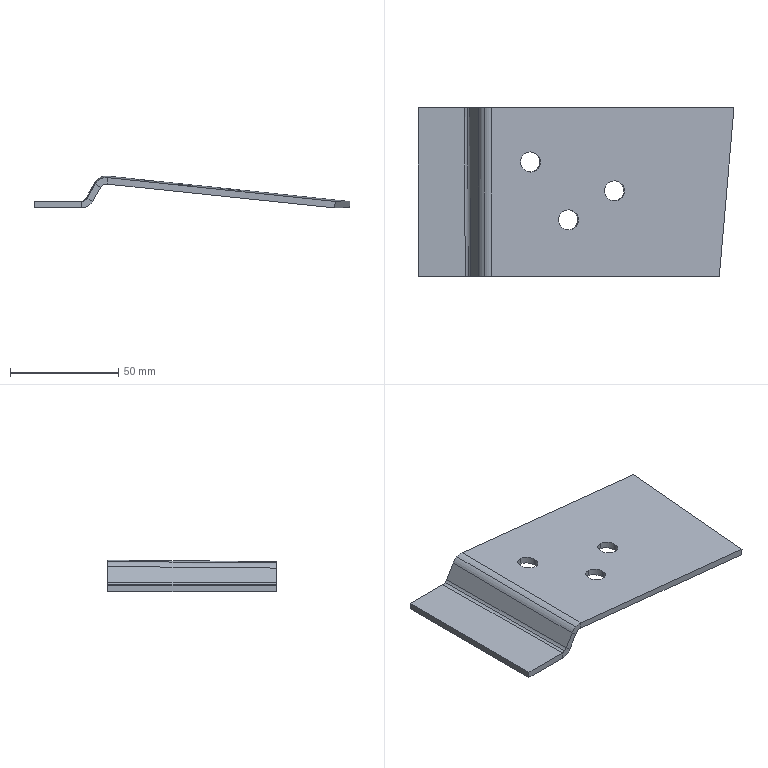Part | NX | features BREP 1 | 1 solid | 38 faces | box 145.982 x 77.757 x 14.741 mm | volume 34048 mm3 | cylinder 20 | plane 14 | spline 4 | commonest cylinder face diameters 9.3 x12 6 x4 12 x4
STEP:
#1=CARTESIAN_POINT('',(747.036,-96.197,42.475));
#2=VERTEX_POINT('',#1);
#3=CARTESIAN_POINT('',(751.661,-91.543,42.034));
#4=VERTEX_POINT('',#3);
#5=CARTESIAN_POINT('',(751.661,-91.543,42.034));
#6=CARTESIAN_POINT('',(751.661,-92.763,42.023));
#7=CARTESIAN_POINT('',(750.656,-95.185,42.106));
#8=CARTESIAN_POINT('',(748.251,-96.196,42.348));
#9=CARTESIAN_POINT('',(747.036,-96.197,42.475));
#10=B_SPLINE_CURVE_WITH_KNOTS('',3,(#5,#6,#7,#8,#9),.UNSPECIFIED.,.F.,.F.,(4,1,4),(0.,0.5,1.),.UNSPECIFIED.);
#11=EDGE_CURVE('',#2,#4,#10,.F.);
#12=ORIENTED_EDGE('',*,*,#11,.T.);
#13=CARTESIAN_POINT('',(751.348,-91.516,39.05));
#14=VERTEX_POINT('',#13);
#15=CARTESIAN_POINT('',(751.348,-91.516,39.05));
#16=DIRECTION('',(0.1041,-0.00911,0.9945));
#17=VECTOR('',#16,1000.);
#18=LINE('',#15,#17);
#19=EDGE_CURVE('',#14,#4,#18,.T.);
#20=ORIENTED_EDGE('',*,*,#19,.F.);
#21=CARTESIAN_POINT('',(746.724,-96.17,39.492));
#22=VERTEX_POINT('',#21);
#23=CARTESIAN_POINT('',(746.724,-96.17,39.492));
#24=CARTESIAN_POINT('',(747.938,-96.169,39.365));
#25=CARTESIAN_POINT('',(750.345,-95.156,39.122));
#26=CARTESIAN_POINT('',(751.348,-92.738,39.039));
#27=CARTESIAN_POINT('',(751.348,-91.516,39.05));
#28=B_SPLINE_CURVE_WITH_KNOTS('',3,(#23,#24,#25,#26,#27),.UNSPECIFIED.,.F.,.F.,(4,1,4),(0.,0.5,1.),.UNSPECIFIED.);
#29=EDGE_CURVE('',#22,#14,#28,.T.);
#30=ORIENTED_EDGE('',*,*,#29,.F.);
#31=CARTESIAN_POINT('',(746.724,-96.17,39.492));
#32=DIRECTION('',(0.1041,-0.00911,0.9945));
#33=VECTOR('',#32,1000.);
#34=LINE('',#31,#33);
#35=EDGE_CURVE('',#22,#2,#34,.T.);
#36=ORIENTED_EDGE('',*,*,#35,.T.);
#37=EDGE_LOOP('',(#12,#20,#30,#36));
#38=FACE_BOUND('',#37,.T.);
#39=CARTESIAN_POINT('',(746.724,-91.52,39.534));
#40=DIRECTION('',(0.1041,-0.00911,0.9945));
#41=DIRECTION('',(0.,-1.,-0.00916));
#42=AXIS2_PLACEMENT_3D('',#39,#40,#41);
#43=CYLINDRICAL_SURFACE('',#42,4.65);
#44=ADVANCED_FACE('',(#38),#43,.F.);
#45=CARTESIAN_POINT('',(742.099,-91.525,40.019));
#46=VERTEX_POINT('',#45);
#47=CARTESIAN_POINT('',(742.099,-91.525,40.019));
#48=CARTESIAN_POINT('',(742.099,-92.745,40.007));
#49=CARTESIAN_POINT('',(743.103,-95.164,39.88));
#50=CARTESIAN_POINT('',(745.508,-96.171,39.619));
#51=CARTESIAN_POINT('',(746.724,-96.17,39.492));
#52=B_SPLINE_CURVE_WITH_KNOTS('',3,(#47,#48,#49,#50,#51),.UNSPECIFIED.,.F.,.F.,(4,1,4),(0.,0.5,1.),.UNSPECIFIED.);
#53=EDGE_CURVE('',#46,#22,#52,.T.);
#54=ORIENTED_EDGE('',*,*,#53,.F.);
#55=CARTESIAN_POINT('',(742.411,-91.552,43.002));
#56=VERTEX_POINT('',#55);
#57=CARTESIAN_POINT('',(742.099,-91.525,40.019));
#58=DIRECTION('',(0.1041,-0.00911,0.9945));
#59=VECTOR('',#58,1000.);
#60=LINE('',#57,#59);
#61=EDGE_CURVE('',#46,#56,#60,.T.);
#62=ORIENTED_EDGE('',*,*,#61,.T.);
#63=CARTESIAN_POINT('',(747.036,-96.197,42.475));
#64=CARTESIAN_POINT('',(745.822,-96.198,42.603));
#65=CARTESIAN_POINT('',(743.415,-95.191,42.864));
#66=CARTESIAN_POINT('',(742.411,-92.774,42.991));
#67=CARTESIAN_POINT('',(742.411,-91.552,43.002));
#68=B_SPLINE_CURVE_WITH_KNOTS('',3,(#63,#64,#65,#66,#67),.UNSPECIFIED.,.F.,.F.,(4,1,4),(0.,0.5,1.),.UNSPECIFIED.);
#69=EDGE_CURVE('',#56,#2,#68,.F.);
#70=ORIENTED_EDGE('',*,*,#69,.T.);
#71=ORIENTED_EDGE('',*,*,#35,.F.);
#72=EDGE_LOOP('',(#54,#62,#70,#71));
#73=FACE_BOUND('',#72,.T.);
#74=CARTESIAN_POINT('',(746.724,-91.52,39.534));
#75=DIRECTION('',(0.1041,-0.00911,0.9945));
#76=DIRECTION('',(0.,1.,0.00916));
#77=AXIS2_PLACEMENT_3D('',#74,#75,#76);
#78=CYLINDRICAL_SURFACE('',#77,4.65);
#79=ADVANCED_FACE('',(#73),#78,.F.);
#80=CARTESIAN_POINT('',(747.036,-86.898,42.561));
#81=VERTEX_POINT('',#80);
#82=CARTESIAN_POINT('',(742.411,-91.552,43.002));
#83=CARTESIAN_POINT('',(742.411,-90.331,43.013));
#84=CARTESIAN_POINT('',(743.416,-87.91,42.93));
#85=CARTESIAN_POINT('',(745.821,-86.899,42.688));
#86=CARTESIAN_POINT('',(747.036,-86.898,42.561));
#87=B_SPLINE_CURVE_WITH_KNOTS('',3,(#82,#83,#84,#85,#86),.UNSPECIFIED.,.F.,.F.,(4,1,4),(0.,0.5,1.),.UNSPECIFIED.);
#88=EDGE_CURVE('',#81,#56,#87,.F.);
#89=ORIENTED_EDGE('',*,*,#88,.T.);
#90=ORIENTED_EDGE('',*,*,#61,.F.);
#91=CARTESIAN_POINT('',(746.724,-86.87,39.577));
#92=VERTEX_POINT('',#91);
#93=CARTESIAN_POINT('',(746.724,-86.87,39.577));
#94=CARTESIAN_POINT('',(745.51,-86.871,39.704));
#95=CARTESIAN_POINT('',(743.103,-87.884,39.947));
#96=CARTESIAN_POINT('',(742.099,-90.303,40.03));
#97=CARTESIAN_POINT('',(742.099,-91.525,40.019));
#98=B_SPLINE_CURVE_WITH_KNOTS('',3,(#93,#94,#95,#96,#97),.UNSPECIFIED.,.F.,.F.,(4,1,4),(0.,0.5,1.),.UNSPECIFIED.);
#99=EDGE_CURVE('',#92,#46,#98,.T.);
#100=ORIENTED_EDGE('',*,*,#99,.F.);
#101=CARTESIAN_POINT('',(746.724,-86.87,39.577));
#102=DIRECTION('',(0.1041,-0.00911,0.9945));
#103=VECTOR('',#102,1000.);
#104=LINE('',#101,#103);
#105=EDGE_CURVE('',#92,#81,#104,.T.);
#106=ORIENTED_EDGE('',*,*,#105,.T.);
#107=EDGE_LOOP('',(#89,#90,#100,#106));
#108=FACE_BOUND('',#107,.T.);
#109=CARTESIAN_POINT('',(746.724,-91.52,39.534));
#110=DIRECTION('',(0.1041,-0.00911,0.9945));
#111=DIRECTION('',(0.,1.,0.00916));
#112=AXIS2_PLACEMENT_3D('',#109,#110,#111);
#113=CYLINDRICAL_SURFACE('',#112,4.65);
#114=ADVANCED_FACE('',(#108),#113,.F.);
#115=CARTESIAN_POINT('',(751.348,-91.516,39.05));
#116=CARTESIAN_POINT('',(751.348,-90.295,39.061));
#117=CARTESIAN_POINT('',(750.344,-87.876,39.189));
#118=CARTESIAN_POINT('',(747.939,-86.869,39.45));
#119=CARTESIAN_POINT('',(746.724,-86.87,39.577));
#120=B_SPLINE_CURVE_WITH_KNOTS('',3,(#115,#116,#117,#118,#119),.UNSPECIFIED.,.F.,.F.,(4,1,4),(0.,0.5,1.),.UNSPECIFIED.);
#121=EDGE_CURVE('',#14,#92,#120,.T.);
#122=ORIENTED_EDGE('',*,*,#121,.F.);
#123=ORIENTED_EDGE('',*,*,#19,.T.);
#124=CARTESIAN_POINT('',(747.036,-86.898,42.561));
#125=CARTESIAN_POINT('',(748.25,-86.896,42.434));
#126=CARTESIAN_POINT('',(750.657,-87.904,42.172));
#127=CARTESIAN_POINT('',(751.661,-90.321,42.045));
#128=CARTESIAN_POINT('',(751.661,-91.543,42.034));
#129=B_SPLINE_CURVE_WITH_KNOTS('',3,(#124,#125,#126,#127,#128),.UNSPECIFIED.,.F.,.F.,(4,1,4),(0.,0.5,1.),.UNSPECIFIED.);
#130=EDGE_CURVE('',#4,#81,#129,.F.);
#131=ORIENTED_EDGE('',*,*,#130,.T.);
#132=ORIENTED_EDGE('',*,*,#105,.F.);
#133=EDGE_LOOP('',(#122,#123,#131,#132));
#134=FACE_BOUND('',#133,.T.);
#135=CARTESIAN_POINT('',(746.724,-91.52,39.534));
#136=DIRECTION('',(0.1041,-0.00911,0.9945));
#137=DIRECTION('',(0.,-1.,-0.00916));
#138=AXIS2_PLACEMENT_3D('',#135,#136,#137);
#139=CYLINDRICAL_SURFACE('',#138,4.65);
#140=ADVANCED_FACE('',(#134),#139,.F.);
#141=CARTESIAN_POINT('',(768.275,-82.797,40.374));
#142=VERTEX_POINT('',#141);
#143=CARTESIAN_POINT('',(772.899,-78.143,39.933));
#144=VERTEX_POINT('',#143);
#145=CARTESIAN_POINT('',(772.899,-78.143,39.933));
#146=CARTESIAN_POINT('',(772.899,-79.364,39.922));
#147=CARTESIAN_POINT('',(771.895,-81.785,40.005));
#148=CARTESIAN_POINT('',(769.49,-82.796,40.247));
#149=CARTESIAN_POINT('',(768.275,-82.797,40.374));
#150=B_SPLINE_CURVE_WITH_KNOTS('',3,(#145,#146,#147,#148,#149),.UNSPECIFIED.,.F.,.F.,(4,1,4),(0.,0.5,1.),.UNSPECIFIED.);
#151=EDGE_CURVE('',#142,#144,#150,.F.);
#152=ORIENTED_EDGE('',*,*,#151,.T.);
#153=CARTESIAN_POINT('',(772.587,-78.116,36.949));
#154=VERTEX_POINT('',#153);
#155=CARTESIAN_POINT('',(772.587,-78.116,36.949));
#156=DIRECTION('',(0.1041,-0.00911,0.9945));
#157=VECTOR('',#156,1000.);
#158=LINE('',#155,#157);
#159=EDGE_CURVE('',#154,#144,#158,.T.);
#160=ORIENTED_EDGE('',*,*,#159,.F.);
#161=CARTESIAN_POINT('',(767.962,-82.77,37.391));
#162=VERTEX_POINT('',#161);
#163=CARTESIAN_POINT('',(767.962,-78.12,37.433));
#164=DIRECTION('',(0.1041,-0.00911,0.9945));
#165=DIRECTION('',(-0.9946,-0.0009538,0.1041));
#166=AXIS2_PLACEMENT_3D('',#163,#164,#165);
#167=CIRCLE('',#166,4.65);
#168=EDGE_CURVE('',#162,#154,#167,.T.);
#169=ORIENTED_EDGE('',*,*,#168,.F.);
#170=CARTESIAN_POINT('',(767.962,-82.77,37.391));
#171=DIRECTION('',(0.1041,-0.00911,0.9945));
#172=VECTOR('',#171,1000.);
#173=LINE('',#170,#172);
#174=EDGE_CURVE('',#162,#142,#173,.T.);
#175=ORIENTED_EDGE('',*,*,#174,.T.);
#176=EDGE_LOOP('',(#152,#160,#169,#175));
#177=FACE_BOUND('',#176,.T.);
#178=CARTESIAN_POINT('',(767.962,-78.12,37.433));
#179=DIRECTION('',(0.1041,-0.00911,0.9945));
#180=DIRECTION('',(0.,-1.,-0.00916));
#181=AXIS2_PLACEMENT_3D('',#178,#179,#180);
#182=CYLINDRICAL_SURFACE('',#181,4.65);
#183=ADVANCED_FACE('',(#177),#182,.F.);
#184=CARTESIAN_POINT('',(763.337,-78.125,37.918));
#185=VERTEX_POINT('',#184);
#186=CARTESIAN_POINT('',(767.962,-78.12,37.433));
#187=DIRECTION('',(0.1041,-0.00911,0.9945));
#188=DIRECTION('',(-0.9946,-0.0009538,0.1041));
#189=AXIS2_PLACEMENT_3D('',#186,#187,#188);
#190=CIRCLE('',#189,4.65);
#191=EDGE_CURVE('',#185,#162,#190,.T.);
#192=ORIENTED_EDGE('',*,*,#191,.F.);
#193=CARTESIAN_POINT('',(763.65,-78.152,40.901));
#194=VERTEX_POINT('',#193);
#195=CARTESIAN_POINT('',(763.337,-78.125,37.918));
#196=DIRECTION('',(0.1041,-0.00911,0.9945));
#197=VECTOR('',#196,1000.);
#198=LINE('',#195,#197);
#199=EDGE_CURVE('',#185,#194,#198,.T.);
#200=ORIENTED_EDGE('',*,*,#199,.T.);
#201=CARTESIAN_POINT('',(768.275,-82.797,40.374));
#202=CARTESIAN_POINT('',(767.061,-82.798,40.501));
#203=CARTESIAN_POINT('',(764.654,-81.791,40.763));
#204=CARTESIAN_POINT('',(763.65,-79.374,40.89));
#205=CARTESIAN_POINT('',(763.65,-78.152,40.901));
#206=B_SPLINE_CURVE_WITH_KNOTS('',3,(#201,#202,#203,#204,#205),.UNSPECIFIED.,.F.,.F.,(4,1,4),(0.,0.5,1.),.UNSPECIFIED.);
#207=EDGE_CURVE('',#194,#142,#206,.F.);
#208=ORIENTED_EDGE('',*,*,#207,.T.);
#209=ORIENTED_EDGE('',*,*,#174,.F.);
#210=EDGE_LOOP('',(#192,#200,#208,#209));
#211=FACE_BOUND('',#210,.T.);
#212=CARTESIAN_POINT('',(767.962,-78.12,37.433));
#213=DIRECTION('',(0.1041,-0.00911,0.9945));
#214=DIRECTION('',(0.,1.,0.00916));
#215=AXIS2_PLACEMENT_3D('',#212,#213,#214);
#216=CYLINDRICAL_SURFACE('',#215,4.65);
#217=ADVANCED_FACE('',(#211),#216,.F.);
#218=CARTESIAN_POINT('',(768.275,-73.498,40.46));
#219=VERTEX_POINT('',#218);
#220=CARTESIAN_POINT('',(763.65,-78.152,40.901));
#221=CARTESIAN_POINT('',(763.65,-76.931,40.912));
#222=CARTESIAN_POINT('',(764.654,-74.51,40.829));
#223=CARTESIAN_POINT('',(767.059,-73.499,40.587));
#224=CARTESIAN_POINT('',(768.275,-73.498,40.46));
#225=B_SPLINE_CURVE_WITH_KNOTS('',3,(#220,#221,#222,#223,#224),.UNSPECIFIED.,.F.,.F.,(4,1,4),(0.,0.5,1.),.UNSPECIFIED.);
#226=EDGE_CURVE('',#219,#194,#225,.F.);
#227=ORIENTED_EDGE('',*,*,#226,.T.);
#228=ORIENTED_EDGE('',*,*,#199,.F.);
#229=CARTESIAN_POINT('',(767.962,-73.47,37.476));
#230=VERTEX_POINT('',#229);
#231=CARTESIAN_POINT('',(767.962,-78.12,37.433));
#232=DIRECTION('',(0.1041,-0.00911,0.9945));
#233=DIRECTION('',(-0.9946,-0.0009538,0.1041));
#234=AXIS2_PLACEMENT_3D('',#231,#232,#233);
#235=CIRCLE('',#234,4.65);
#236=EDGE_CURVE('',#230,#185,#235,.T.);
#237=ORIENTED_EDGE('',*,*,#236,.F.);
#238=CARTESIAN_POINT('',(767.962,-73.47,37.476));
#239=DIRECTION('',(0.1041,-0.00911,0.9945));
#240=VECTOR('',#239,1000.);
#241=LINE('',#238,#240);
#242=EDGE_CURVE('',#230,#219,#241,.T.);
#243=ORIENTED_EDGE('',*,*,#242,.T.);
#244=EDGE_LOOP('',(#227,#228,#237,#243));
#245=FACE_BOUND('',#244,.T.);
#246=CARTESIAN_POINT('',(767.962,-78.12,37.433));
#247=DIRECTION('',(0.1041,-0.00911,0.9945));
#248=DIRECTION('',(0.,1.,0.00916));
#249=AXIS2_PLACEMENT_3D('',#246,#247,#248);
#250=CYLINDRICAL_SURFACE('',#249,4.65);
#251=ADVANCED_FACE('',(#245),#250,.F.);
#252=CARTESIAN_POINT('',(767.962,-78.12,37.433));
#253=DIRECTION('',(0.1041,-0.00911,0.9945));
#254=DIRECTION('',(-0.9946,-0.0009538,0.1041));
#255=AXIS2_PLACEMENT_3D('',#252,#253,#254);
#256=CIRCLE('',#255,4.65);
#257=EDGE_CURVE('',#154,#230,#256,.T.);
#258=ORIENTED_EDGE('',*,*,#257,.F.);
#259=ORIENTED_EDGE('',*,*,#159,.T.);
#260=CARTESIAN_POINT('',(768.275,-73.498,40.46));
#261=CARTESIAN_POINT('',(769.489,-73.497,40.332));
#262=CARTESIAN_POINT('',(771.896,-74.504,40.071));
#263=CARTESIAN_POINT('',(772.899,-76.921,39.944));
#264=CARTESIAN_POINT('',(772.899,-78.143,39.933));
#265=B_SPLINE_CURVE_WITH_KNOTS('',3,(#260,#261,#262,#263,#264),.UNSPECIFIED.,.F.,.F.,(4,1,4),(0.,0.5,1.),.UNSPECIFIED.);
#266=EDGE_CURVE('',#144,#219,#265,.F.);
#267=ORIENTED_EDGE('',*,*,#266,.T.);
#268=ORIENTED_EDGE('',*,*,#242,.F.);
#269=EDGE_LOOP('',(#258,#259,#267,#268));
#270=FACE_BOUND('',#269,.T.);
#271=CARTESIAN_POINT('',(767.962,-78.12,37.433));
#272=DIRECTION('',(0.1041,-0.00911,0.9945));
#273=DIRECTION('',(0.,-1.,-0.00916));
#274=AXIS2_PLACEMENT_3D('',#271,#272,#273);
#275=CYLINDRICAL_SURFACE('',#274,4.65);
#276=ADVANCED_FACE('',(#270),#275,.F.);
#277=CARTESIAN_POINT('',(729.508,-69.468,44.556));
#278=VERTEX_POINT('',#277);
#279=CARTESIAN_POINT('',(734.133,-64.814,44.114));
#280=VERTEX_POINT('',#279);
#281=CARTESIAN_POINT('',(734.133,-64.814,44.114));
#282=CARTESIAN_POINT('',(734.133,-66.034,44.103));
#283=CARTESIAN_POINT('',(733.128,-68.455,44.186));
#284=CARTESIAN_POINT('',(730.723,-69.467,44.428));
#285=CARTESIAN_POINT('',(729.508,-69.468,44.556));
#286=B_SPLINE_CURVE_WITH_KNOTS('',3,(#281,#282,#283,#284,#285),.UNSPECIFIED.,.F.,.F.,(4,1,4),(0.,0.5,1.),.UNSPECIFIED.);
#287=EDGE_CURVE('',#278,#280,#286,.F.);
#288=ORIENTED_EDGE('',*,*,#287,.T.);
#289=CARTESIAN_POINT('',(733.82,-64.786,41.13));
#290=VERTEX_POINT('',#289);
#291=CARTESIAN_POINT('',(733.82,-64.786,41.13));
#292=DIRECTION('',(0.1041,-0.00911,0.9945));
#293=VECTOR('',#292,1000.);
#294=LINE('',#291,#293);
#295=EDGE_CURVE('',#290,#280,#294,.T.);
#296=ORIENTED_EDGE('',*,*,#295,.F.);
#297=CARTESIAN_POINT('',(729.196,-69.441,41.572));
#298=VERTEX_POINT('',#297);
#299=CARTESIAN_POINT('',(729.196,-69.441,41.572));
#300=CARTESIAN_POINT('',(730.41,-69.439,41.445));
#301=CARTESIAN_POINT('',(732.817,-68.427,41.202));
#302=CARTESIAN_POINT('',(733.82,-66.008,41.119));
#303=CARTESIAN_POINT('',(733.82,-64.786,41.13));
#304=B_SPLINE_CURVE_WITH_KNOTS('',3,(#299,#300,#301,#302,#303),.UNSPECIFIED.,.F.,.F.,(4,1,4),(0.,0.5,1.),.UNSPECIFIED.);
#305=EDGE_CURVE('',#298,#290,#304,.T.);
#306=ORIENTED_EDGE('',*,*,#305,.F.);
#307=CARTESIAN_POINT('',(729.196,-69.441,41.572));
#308=DIRECTION('',(0.1041,-0.00911,0.9945));
#309=VECTOR('',#308,1000.);
#310=LINE('',#307,#309);
#311=EDGE_CURVE('',#298,#278,#310,.T.);
#312=ORIENTED_EDGE('',*,*,#311,.T.);
#313=EDGE_LOOP('',(#288,#296,#306,#312));
#314=FACE_BOUND('',#313,.T.);
#315=CARTESIAN_POINT('',(729.196,-64.791,41.615));
#316=DIRECTION('',(0.1041,-0.00911,0.9945));
#317=DIRECTION('',(0.,-1.,-0.00916));
#318=AXIS2_PLACEMENT_3D('',#315,#316,#317);
#319=CYLINDRICAL_SURFACE('',#318,4.65);
#320=ADVANCED_FACE('',(#314),#319,.F.);
#321=CARTESIAN_POINT('',(724.571,-64.795,42.099));
#322=VERTEX_POINT('',#321);
#323=CARTESIAN_POINT('',(724.571,-64.795,42.099));
#324=CARTESIAN_POINT('',(724.571,-66.016,42.088));
#325=CARTESIAN_POINT('',(725.575,-68.435,41.96));
#326=CARTESIAN_POINT('',(727.98,-69.442,41.699));
#327=CARTESIAN_POINT('',(729.196,-69.441,41.572));
#328=B_SPLINE_CURVE_WITH_KNOTS('',3,(#323,#324,#325,#326,#327),.UNSPECIFIED.,.F.,.F.,(4,1,4),(0.,0.5,1.),.UNSPECIFIED.);
#329=EDGE_CURVE('',#322,#298,#328,.T.);
#330=ORIENTED_EDGE('',*,*,#329,.F.);
#331=CARTESIAN_POINT('',(724.883,-64.822,45.082));
#332=VERTEX_POINT('',#331);
#333=CARTESIAN_POINT('',(724.571,-64.795,42.099));
#334=DIRECTION('',(0.1041,-0.00911,0.9945));
#335=VECTOR('',#334,1000.);
#336=LINE('',#333,#335);
#337=EDGE_CURVE('',#322,#332,#336,.T.);
#338=ORIENTED_EDGE('',*,*,#337,.T.);
#339=CARTESIAN_POINT('',(729.508,-69.468,44.556));
#340=CARTESIAN_POINT('',(728.294,-69.469,44.683));
#341=CARTESIAN_POINT('',(725.887,-68.461,44.944));
#342=CARTESIAN_POINT('',(724.883,-66.044,45.071));
#343=CARTESIAN_POINT('',(724.883,-64.822,45.082));
#344=B_SPLINE_CURVE_WITH_KNOTS('',3,(#339,#340,#341,#342,#343),.UNSPECIFIED.,.F.,.F.,(4,1,4),(0.,0.5,1.),.UNSPECIFIED.);
#345=EDGE_CURVE('',#332,#278,#344,.F.);
#346=ORIENTED_EDGE('',*,*,#345,.T.);
#347=ORIENTED_EDGE('',*,*,#311,.F.);
#348=EDGE_LOOP('',(#330,#338,#346,#347));
#349=FACE_BOUND('',#348,.T.);
#350=CARTESIAN_POINT('',(729.196,-64.791,41.615));
#351=DIRECTION('',(0.1041,-0.00911,0.9945));
#352=DIRECTION('',(0.,1.,0.00916));
#353=AXIS2_PLACEMENT_3D('',#350,#351,#352);
#354=CYLINDRICAL_SURFACE('',#353,4.65);
#355=ADVANCED_FACE('',(#349),#354,.F.);
#356=CARTESIAN_POINT('',(729.508,-60.168,44.641));
#357=VERTEX_POINT('',#356);
#358=CARTESIAN_POINT('',(724.883,-64.822,45.082));
#359=CARTESIAN_POINT('',(724.883,-63.602,45.093));
#360=CARTESIAN_POINT('',(725.888,-61.181,45.011));
#361=CARTESIAN_POINT('',(728.293,-60.169,44.768));
#362=CARTESIAN_POINT('',(729.508,-60.168,44.641));
#363=B_SPLINE_CURVE_WITH_KNOTS('',3,(#358,#359,#360,#361,#362),.UNSPECIFIED.,.F.,.F.,(4,1,4),(0.,0.5,1.),.UNSPECIFIED.);
#364=EDGE_CURVE('',#357,#332,#363,.F.);
#365=ORIENTED_EDGE('',*,*,#364,.T.);
#366=ORIENTED_EDGE('',*,*,#337,.F.);
#367=CARTESIAN_POINT('',(729.196,-60.141,41.657));
#368=VERTEX_POINT('',#367);
#369=CARTESIAN_POINT('',(729.196,-60.141,41.657));
#370=CARTESIAN_POINT('',(727.982,-60.142,41.784));
#371=CARTESIAN_POINT('',(725.574,-61.154,42.027));
#372=CARTESIAN_POINT('',(724.571,-63.573,42.11));
#373=CARTESIAN_POINT('',(724.571,-64.795,42.099));
#374=B_SPLINE_CURVE_WITH_KNOTS('',3,(#369,#370,#371,#372,#373),.UNSPECIFIED.,.F.,.F.,(4,1,4),(0.,0.5,1.),.UNSPECIFIED.);
#375=EDGE_CURVE('',#368,#322,#374,.T.);
#376=ORIENTED_EDGE('',*,*,#375,.F.);
#377=CARTESIAN_POINT('',(729.196,-60.141,41.657));
#378=DIRECTION('',(0.1041,-0.00911,0.9945));
#379=VECTOR('',#378,1000.);
#380=LINE('',#377,#379);
#381=EDGE_CURVE('',#368,#357,#380,.T.);
#382=ORIENTED_EDGE('',*,*,#381,.T.);
#383=EDGE_LOOP('',(#365,#366,#376,#382));
#384=FACE_BOUND('',#383,.T.);
#385=CARTESIAN_POINT('',(729.196,-64.791,41.615));
#386=DIRECTION('',(0.1041,-0.00911,0.9945));
#387=DIRECTION('',(0.,1.,0.00916));
#388=AXIS2_PLACEMENT_3D('',#385,#386,#387);
#389=CYLINDRICAL_SURFACE('',#388,4.65);
#390=ADVANCED_FACE('',(#384),#389,.F.);
#391=CARTESIAN_POINT('',(733.82,-64.786,41.13));
#392=CARTESIAN_POINT('',(733.82,-63.566,41.142));
#393=CARTESIAN_POINT('',(732.816,-61.147,41.269));
#394=CARTESIAN_POINT('',(730.411,-60.14,41.53));
#395=CARTESIAN_POINT('',(729.196,-60.141,41.657));
#396=B_SPLINE_CURVE_WITH_KNOTS('',3,(#391,#392,#393,#394,#395),.UNSPECIFIED.,.F.,.F.,(4,1,4),(0.,0.5,1.),.UNSPECIFIED.);
#397=EDGE_CURVE('',#290,#368,#396,.T.);
#398=ORIENTED_EDGE('',*,*,#397,.F.);
#399=ORIENTED_EDGE('',*,*,#295,.T.);
#400=CARTESIAN_POINT('',(729.508,-60.168,44.641));
#401=CARTESIAN_POINT('',(730.722,-60.167,44.514));
#402=CARTESIAN_POINT('',(733.129,-61.175,44.252));
#403=CARTESIAN_POINT('',(734.133,-63.592,44.125));
#404=CARTESIAN_POINT('',(734.133,-64.814,44.114));
#405=B_SPLINE_CURVE_WITH_KNOTS('',3,(#400,#401,#402,#403,#404),.UNSPECIFIED.,.F.,.F.,(4,1,4),(0.,0.5,1.),.UNSPECIFIED.);
#406=EDGE_CURVE('',#280,#357,#405,.F.);
#407=ORIENTED_EDGE('',*,*,#406,.T.);
#408=ORIENTED_EDGE('',*,*,#381,.F.);
#409=EDGE_LOOP('',(#398,#399,#407,#408));
#410=FACE_BOUND('',#409,.T.);
#411=CARTESIAN_POINT('',(729.196,-64.791,41.615));
#412=DIRECTION('',(0.1041,-0.00911,0.9945));
#413=DIRECTION('',(0.,-1.,-0.00916));
#414=AXIS2_PLACEMENT_3D('',#411,#412,#413);
#415=CYLINDRICAL_SURFACE('',#414,4.65);
#416=ADVANCED_FACE('',(#410),#415,.F.);
#417=CARTESIAN_POINT('',(711.225,-39.791,43.725));
#418=VERTEX_POINT('',#417);
#419=CARTESIAN_POINT('',(823.208,-39.791,32.));
#420=VERTEX_POINT('',#419);
#421=CARTESIAN_POINT('',(767.216,-39.791,37.863));
#422=DIRECTION('',(0.9946,0.,-0.1041));
#423=VECTOR('',#422,1000.);
#424=LINE('',#421,#423);
#425=EDGE_CURVE('',#418,#420,#424,.T.);
#426=ORIENTED_EDGE('',*,*,#425,.F.);
#427=CARTESIAN_POINT('',(711.537,-39.818,46.709));
#428=VERTEX_POINT('',#427);
#429=CARTESIAN_POINT('',(711.225,-39.791,43.725));
#430=CARTESIAN_POINT('',(711.537,-39.818,46.709));
#431=B_SPLINE_CURVE_WITH_KNOTS('',1,(#429,#430),.UNSPECIFIED.,.F.,.F.,(2,2),(0.,3.008),.UNSPECIFIED.);
#432=EDGE_CURVE('',#418,#428,#431,.T.);
#433=ORIENTED_EDGE('',*,*,#432,.T.);
#434=CARTESIAN_POINT('',(823.52,-39.818,34.984));
#435=VERTEX_POINT('',#434);
#436=CARTESIAN_POINT('',(767.529,-39.818,40.846));
#437=DIRECTION('',(0.9946,0.,-0.1041));
#438=VECTOR('',#437,1000.);
#439=LINE('',#436,#438);
#440=EDGE_CURVE('',#428,#435,#439,.T.);
#441=ORIENTED_EDGE('',*,*,#440,.T.);
#442=CARTESIAN_POINT('',(823.364,-39.804,33.492));
#443=DIRECTION('',(0.1041,-0.00911,0.9945));
#444=VECTOR('',#443,1000.);
#445=LINE('',#442,#444);
#446=EDGE_CURVE('',#420,#435,#445,.T.);
#447=ORIENTED_EDGE('',*,*,#446,.F.);
#448=EDGE_LOOP('',(#426,#433,#441,#447));
#449=FACE_BOUND('',#448,.T.);
#450=CARTESIAN_POINT('',(767.216,-39.791,37.863));
#451=DIRECTION('',(0.0009487,1.,0.009061));
#452=DIRECTION('',(1.,-0.0009487,-0.000008596));
#453=AXIS2_PLACEMENT_3D('',#450,#451,#452);
#454=PLANE('',#453);
#455=ADVANCED_FACE('',(#449),#454,.T.);
#456=ORIENTED_EDGE('',*,*,#11,.F.);
#457=ORIENTED_EDGE('',*,*,#69,.F.);
#458=ORIENTED_EDGE('',*,*,#88,.F.);
#459=ORIENTED_EDGE('',*,*,#130,.F.);
#460=EDGE_LOOP('',(#456,#457,#458,#459));
#461=FACE_BOUND('',#460,.T.);
#462=ORIENTED_EDGE('',*,*,#151,.F.);
#463=ORIENTED_EDGE('',*,*,#207,.F.);
#464=ORIENTED_EDGE('',*,*,#226,.F.);
#465=ORIENTED_EDGE('',*,*,#266,.F.);
#466=EDGE_LOOP('',(#462,#463,#464,#465));
#467=FACE_BOUND('',#466,.T.);
#468=ORIENTED_EDGE('',*,*,#287,.F.);
#469=ORIENTED_EDGE('',*,*,#345,.F.);
#470=ORIENTED_EDGE('',*,*,#364,.F.);
#471=ORIENTED_EDGE('',*,*,#406,.F.);
#472=EDGE_LOOP('',(#468,#469,#470,#471));
#473=FACE_BOUND('',#472,.T.);
#474=CARTESIAN_POINT('',(816.72,-117.547,34.984));
#475=VERTEX_POINT('',#474);
#476=CARTESIAN_POINT('',(820.12,-78.683,34.984));
#477=DIRECTION('',(0.08716,0.9962,0.));
#478=VECTOR('',#477,1000.);
#479=LINE('',#476,#478);
#480=EDGE_CURVE('',#475,#435,#479,.T.);
#481=ORIENTED_EDGE('',*,*,#480,.T.);
#482=ORIENTED_EDGE('',*,*,#440,.F.);
#483=CARTESIAN_POINT('',(711.537,-117.547,45.997));
#484=VERTEX_POINT('',#483);
#485=CARTESIAN_POINT('',(711.537,-75.45,46.382));
#486=DIRECTION('',(0.,1.,0.00916));
#487=VECTOR('',#486,1000.);
#488=LINE('',#485,#487);
#489=EDGE_CURVE('',#484,#428,#488,.T.);
#490=ORIENTED_EDGE('',*,*,#489,.F.);
#491=CARTESIAN_POINT('',(764.128,-117.547,40.49));
#492=DIRECTION('',(0.9946,0.,-0.1041));
#493=VECTOR('',#492,1000.);
#494=LINE('',#491,#493);
#495=EDGE_CURVE('',#484,#475,#494,.T.);
#496=ORIENTED_EDGE('',*,*,#495,.T.);
#497=EDGE_LOOP('',(#481,#482,#490,#496));
#498=FACE_BOUND('',#497,.T.);
#499=CARTESIAN_POINT('',(757.353,-84.219,41.505));
#500=DIRECTION('',(0.1041,-0.00911,0.9945));
#501=DIRECTION('',(0.9907,-0.08668,-0.1045));
#502=AXIS2_PLACEMENT_3D('',#499,#500,#501);
#503=PLANE('',#502);
#504=ADVANCED_FACE('',(#461,#467,#473,#498),#503,.T.);
#505=CARTESIAN_POINT('',(816.407,-117.52,32.));
#506=VERTEX_POINT('',#505);
#507=CARTESIAN_POINT('',(819.808,-78.655,32.));
#508=DIRECTION('',(0.08716,0.9962,0.));
#509=VECTOR('',#508,1000.);
#510=LINE('',#507,#509);
#511=EDGE_CURVE('',#506,#420,#510,.T.);
#512=ORIENTED_EDGE('',*,*,#511,.T.);
#513=ORIENTED_EDGE('',*,*,#446,.T.);
#514=ORIENTED_EDGE('',*,*,#480,.F.);
#515=CARTESIAN_POINT('',(816.564,-117.534,33.492));
#516=DIRECTION('',(0.1041,-0.00911,0.9945));
#517=VECTOR('',#516,1000.);
#518=LINE('',#515,#517);
#519=EDGE_CURVE('',#506,#475,#518,.T.);
#520=ORIENTED_EDGE('',*,*,#519,.F.);
#521=EDGE_LOOP('',(#512,#513,#514,#520));
#522=FACE_BOUND('',#521,.T.);
#523=CARTESIAN_POINT('',(819.808,-78.655,32.));
#524=DIRECTION('',(0.9907,-0.08668,-0.1045));
#525=DIRECTION('',(0.1358,0.6324,0.7626));
#526=AXIS2_PLACEMENT_3D('',#523,#524,#525);
#527=PLANE('',#526);
#528=ADVANCED_FACE('',(#522),#527,.T.);
#529=ORIENTED_EDGE('',*,*,#121,.T.);
#530=ORIENTED_EDGE('',*,*,#99,.T.);
#531=ORIENTED_EDGE('',*,*,#53,.T.);
#532=ORIENTED_EDGE('',*,*,#29,.T.);
#533=EDGE_LOOP('',(#529,#530,#531,#532));
#534=FACE_BOUND('',#533,.T.);
#535=ORIENTED_EDGE('',*,*,#257,.T.);
#536=ORIENTED_EDGE('',*,*,#236,.T.);
#537=ORIENTED_EDGE('',*,*,#191,.T.);
#538=ORIENTED_EDGE('',*,*,#168,.T.);
#539=EDGE_LOOP('',(#535,#536,#537,#538));
#540=FACE_BOUND('',#539,.T.);
#541=ORIENTED_EDGE('',*,*,#397,.T.);
#542=ORIENTED_EDGE('',*,*,#375,.T.);
#543=ORIENTED_EDGE('',*,*,#329,.T.);
#544=ORIENTED_EDGE('',*,*,#305,.T.);
#545=EDGE_LOOP('',(#541,#542,#543,#544));
#546=FACE_BOUND('',#545,.T.);
#547=CARTESIAN_POINT('',(711.225,-117.52,43.013));
#548=VERTEX_POINT('',#547);
#549=CARTESIAN_POINT('',(763.816,-117.52,37.507));
#550=DIRECTION('',(0.9946,0.,-0.1041));
#551=VECTOR('',#550,1000.);
#552=LINE('',#549,#551);
#553=EDGE_CURVE('',#548,#506,#552,.T.);
#554=ORIENTED_EDGE('',*,*,#553,.F.);
#555=CARTESIAN_POINT('',(711.225,-75.423,43.399));
#556=DIRECTION('',(0.,1.,0.00916));
#557=VECTOR('',#556,1000.);
#558=LINE('',#555,#557);
#559=EDGE_CURVE('',#548,#418,#558,.T.);
#560=ORIENTED_EDGE('',*,*,#559,.T.);
#561=ORIENTED_EDGE('',*,*,#425,.T.);
#562=ORIENTED_EDGE('',*,*,#511,.F.);
#563=EDGE_LOOP('',(#554,#560,#561,#562));
#564=FACE_BOUND('',#563,.T.);
#565=CARTESIAN_POINT('',(757.04,-84.191,38.521));
#566=DIRECTION('',(0.1041,-0.00911,0.9945));
#567=DIRECTION('',(0.9907,-0.08668,-0.1045));
#568=AXIS2_PLACEMENT_3D('',#565,#566,#567);
#569=PLANE('',#568);
#570=ADVANCED_FACE('',(#534,#540,#546,#564),#569,.F.);
#571=CARTESIAN_POINT('',(705.716,-39.818,43.741));
#572=VERTEX_POINT('',#571);
#573=CARTESIAN_POINT('',(708.314,-39.804,42.241));
#574=VERTEX_POINT('',#573);
#575=CARTESIAN_POINT('',(705.716,-39.818,43.741));
#576=CARTESIAN_POINT('',(708.314,-39.804,42.241));
#577=B_SPLINE_CURVE_WITH_KNOTS('',1,(#575,#576),.UNSPECIFIED.,.F.,.F.,(2,2),(-3.,0.),.UNSPECIFIED.);
#578=EDGE_CURVE('',#572,#574,#577,.T.);
#579=ORIENTED_EDGE('',*,*,#578,.F.);
#580=CARTESIAN_POINT('',(708.187,-39.818,46.087));
#581=VERTEX_POINT('',#580);
#582=CARTESIAN_POINT('',(708.187,-39.818,46.087));
#583=CARTESIAN_POINT('',(707.255,-39.818,45.612));
#584=CARTESIAN_POINT('',(706.344,-39.818,44.83));
#585=CARTESIAN_POINT('',(705.716,-39.818,43.741));
#586=B_SPLINE_CURVE_WITH_KNOTS('',3,(#582,#583,#584,#585),.UNSPECIFIED.,.F.,.F.,(4,4),(0.,1.),.UNSPECIFIED.);
#587=EDGE_CURVE('',#581,#572,#586,.T.);
#588=ORIENTED_EDGE('',*,*,#587,.F.);
#589=CARTESIAN_POINT('',(711.537,-39.818,46.709));
#590=CARTESIAN_POINT('',(710.413,-39.818,46.826));
#591=CARTESIAN_POINT('',(709.232,-39.818,46.619));
#592=CARTESIAN_POINT('',(708.187,-39.818,46.087));
#593=B_SPLINE_CURVE_WITH_KNOTS('',3,(#589,#590,#591,#592),.UNSPECIFIED.,.F.,.F.,(4,4),(0.,1.),.UNSPECIFIED.);
#594=EDGE_CURVE('',#428,#581,#593,.T.);
#595=ORIENTED_EDGE('',*,*,#594,.F.);
#596=ORIENTED_EDGE('',*,*,#432,.F.);
#597=CARTESIAN_POINT('',(709.55,-39.794,43.414));
#598=VERTEX_POINT('',#597);
#599=CARTESIAN_POINT('',(709.55,-39.794,43.414));
#600=CARTESIAN_POINT('',(710.072,-39.791,43.68));
#601=CARTESIAN_POINT('',(710.662,-39.79,43.784));
#602=CARTESIAN_POINT('',(711.225,-39.791,43.725));
#603=B_SPLINE_CURVE_WITH_KNOTS('',3,(#599,#600,#601,#602),.UNSPECIFIED.,.F.,.F.,(4,4),(0.,1.),.UNSPECIFIED.);
#604=EDGE_CURVE('',#418,#598,#603,.F.);
#605=ORIENTED_EDGE('',*,*,#604,.T.);
#606=CARTESIAN_POINT('',(708.314,-39.804,42.241));
#607=CARTESIAN_POINT('',(708.602,-39.802,42.74));
#608=CARTESIAN_POINT('',(709.037,-39.798,43.153));
#609=CARTESIAN_POINT('',(709.55,-39.794,43.414));
#610=B_SPLINE_CURVE_WITH_KNOTS('',3,(#606,#607,#608,#609),.UNSPECIFIED.,.F.,.F.,(4,4),(0.,1.),.UNSPECIFIED.);
#611=EDGE_CURVE('',#598,#574,#610,.F.);
#612=ORIENTED_EDGE('',*,*,#611,.T.);
#613=EDGE_LOOP('',(#579,#588,#595,#596,#605,#612));
#614=FACE_BOUND('',#613,.T.);
#615=CARTESIAN_POINT('',(711.225,-39.791,43.725));
#616=CARTESIAN_POINT('',(711.537,-39.818,46.709));
#617=CARTESIAN_POINT('',(711.019,-39.791,43.747));
#618=CARTESIAN_POINT('',(711.125,-39.818,46.752));
#619=CARTESIAN_POINT('',(710.811,-39.79,43.751));
#620=CARTESIAN_POINT('',(710.709,-39.818,46.759));
#621=CARTESIAN_POINT('',(710.603,-39.791,43.736));
#622=CARTESIAN_POINT('',(710.293,-39.818,46.731));
#623=CARTESIAN_POINT('',(710.192,-39.791,43.672));
#624=CARTESIAN_POINT('',(709.471,-39.818,46.603));
#625=CARTESIAN_POINT('',(709.798,-39.792,43.538));
#626=CARTESIAN_POINT('',(708.683,-39.818,46.335));
#627=CARTESIAN_POINT('',(709.607,-39.793,43.455));
#628=CARTESIAN_POINT('',(708.301,-39.818,46.167));
#629=CARTESIAN_POINT('',(709.242,-39.795,43.255));
#630=CARTESIAN_POINT('',(707.571,-39.818,45.768));
#631=CARTESIAN_POINT('',(708.916,-39.797,42.996));
#632=CARTESIAN_POINT('',(706.921,-39.818,45.25));
#633=CARTESIAN_POINT('',(708.765,-39.799,42.852));
#634=CARTESIAN_POINT('',(706.618,-39.818,44.963));
#635=CARTESIAN_POINT('',(708.581,-39.801,42.644));
#636=CARTESIAN_POINT('',(706.25,-39.818,44.547));
#637=CARTESIAN_POINT('',(708.423,-39.803,42.418));
#638=CARTESIAN_POINT('',(705.934,-39.818,44.094));
#639=CARTESIAN_POINT('',(708.385,-39.803,42.36));
#640=CARTESIAN_POINT('',(705.858,-39.818,43.979));
#641=CARTESIAN_POINT('',(708.349,-39.804,42.301));
#642=CARTESIAN_POINT('',(705.785,-39.818,43.861));
#643=CARTESIAN_POINT('',(708.314,-39.804,42.241));
#644=CARTESIAN_POINT('',(705.716,-39.818,43.741));
#645=B_SPLINE_SURFACE_WITH_KNOTS('',5,1,((#615,#616),(#617,#618),(#619,#620),(#621,#622),(#623,#624),(#625,#626),(#627,#628),(#629,#630),(#631,#632),(#633,#634),(#635,#636),(#637,#638),(#639,#640),(#641,#642),(#643,#644)),.RULED_SURF.,.F.,.F.,.F.,(6,3,3,3,6),(2,2),(0.,1.558,3.116,4.674,5.194),(0.,3.008),.UNSPECIFIED.);
#646=ADVANCED_FACE('',(#614),#645,.T.);
#647=CARTESIAN_POINT('',(708.187,-117.547,45.375));
#648=VERTEX_POINT('',#647);
#649=CARTESIAN_POINT('',(708.187,-75.445,45.761));
#650=DIRECTION('',(0.,1.,0.00916));
#651=VECTOR('',#650,1000.);
#652=LINE('',#649,#651);
#653=EDGE_CURVE('',#648,#581,#652,.T.);
#654=ORIENTED_EDGE('',*,*,#653,.T.);
#655=ORIENTED_EDGE('',*,*,#587,.T.);
#656=CARTESIAN_POINT('',(705.716,-117.547,43.029));
#657=VERTEX_POINT('',#656);
#658=CARTESIAN_POINT('',(705.716,-117.547,43.029));
#659=CARTESIAN_POINT('',(705.716,-102.002,43.172));
#660=CARTESIAN_POINT('',(705.716,-86.456,43.314));
#661=CARTESIAN_POINT('',(705.716,-70.91,43.457));
#662=CARTESIAN_POINT('',(705.716,-55.364,43.599));
#663=CARTESIAN_POINT('',(705.716,-39.818,43.741));
#664=B_SPLINE_CURVE_WITH_KNOTS('',5,(#658,#659,#660,#661,#662,#663),.UNSPECIFIED.,.F.,.F.,(6,6),(0.,77.733),.UNSPECIFIED.);
#665=EDGE_CURVE('',#657,#572,#664,.T.);
#666=ORIENTED_EDGE('',*,*,#665,.F.);
#667=CARTESIAN_POINT('',(708.187,-117.547,45.375));
#668=CARTESIAN_POINT('',(708.064,-117.547,45.312));
#669=CARTESIAN_POINT('',(707.943,-117.547,45.246));
#670=CARTESIAN_POINT('',(707.824,-117.547,45.176));
#671=CARTESIAN_POINT('',(707.354,-117.547,44.883));
#672=CARTESIAN_POINT('',(706.921,-117.547,44.538));
#673=CARTESIAN_POINT('',(706.618,-117.547,44.251));
#674=CARTESIAN_POINT('',(706.25,-117.547,43.835));
#675=CARTESIAN_POINT('',(705.934,-117.547,43.382));
#676=CARTESIAN_POINT('',(705.858,-117.547,43.267));
#677=CARTESIAN_POINT('',(705.785,-117.547,43.149));
#678=CARTESIAN_POINT('',(705.716,-117.547,43.029));
#679=B_SPLINE_CURVE_WITH_KNOTS('',5,(#667,#668,#669,#670,#671,#672,#673,#674,#675,#676,#677,#678),.UNSPECIFIED.,.F.,.F.,(6,3,3,6),(2.597,3.116,4.674,5.194),.UNSPECIFIED.);
#680=EDGE_CURVE('',#648,#657,#679,.T.);
#681=ORIENTED_EDGE('',*,*,#680,.F.);
#682=EDGE_LOOP('',(#654,#655,#666,#681));
#683=FACE_BOUND('',#682,.T.);
#684=CARTESIAN_POINT('',(710.912,-75.396,40.415));
#685=DIRECTION('',(0.,1.,0.00916));
#686=DIRECTION('',(0.4542,0.008161,-0.8909));
#687=AXIS2_PLACEMENT_3D('',#684,#685,#686);
#688=CYLINDRICAL_SURFACE('',#687,6.);
#689=ADVANCED_FACE('',(#683),#688,.T.);
#690=ORIENTED_EDGE('',*,*,#653,.F.);
#691=CARTESIAN_POINT('',(711.537,-117.547,45.997));
#692=CARTESIAN_POINT('',(711.125,-117.547,46.04));
#693=CARTESIAN_POINT('',(710.709,-117.547,46.047));
#694=CARTESIAN_POINT('',(710.293,-117.547,46.019));
#695=CARTESIAN_POINT('',(709.608,-117.547,45.912));
#696=CARTESIAN_POINT('',(708.947,-117.547,45.708));
#697=CARTESIAN_POINT('',(708.687,-117.547,45.612));
#698=CARTESIAN_POINT('',(708.434,-117.547,45.5));
#699=CARTESIAN_POINT('',(708.187,-117.547,45.375));
#700=B_SPLINE_CURVE_WITH_KNOTS('',5,(#691,#692,#693,#694,#695,#696,#697,#698,#699),.UNSPECIFIED.,.F.,.F.,(6,3,6),(0.,1.558,2.597),.UNSPECIFIED.);
#701=EDGE_CURVE('',#484,#648,#700,.T.);
#702=ORIENTED_EDGE('',*,*,#701,.F.);
#703=ORIENTED_EDGE('',*,*,#489,.T.);
#704=ORIENTED_EDGE('',*,*,#594,.T.);
#705=EDGE_LOOP('',(#690,#702,#703,#704));
#706=FACE_BOUND('',#705,.T.);
#707=CARTESIAN_POINT('',(710.912,-75.396,40.415));
#708=DIRECTION('',(0.,1.,0.00916));
#709=DIRECTION('',(-0.4542,-0.008161,0.8909));
#710=AXIS2_PLACEMENT_3D('',#707,#708,#709);
#711=CYLINDRICAL_SURFACE('',#710,6.);
#712=ADVANCED_FACE('',(#706),#711,.T.);
#713=ORIENTED_EDGE('',*,*,#519,.T.);
#714=ORIENTED_EDGE('',*,*,#495,.F.);
#715=CARTESIAN_POINT('',(711.225,-117.52,43.013));
#716=CARTESIAN_POINT('',(711.537,-117.547,45.997));
#717=B_SPLINE_CURVE_WITH_KNOTS('',1,(#715,#716),.UNSPECIFIED.,.F.,.F.,(2,2),(0.,3.008),.UNSPECIFIED.);
#718=EDGE_CURVE('',#548,#484,#717,.T.);
#719=ORIENTED_EDGE('',*,*,#718,.F.);
#720=ORIENTED_EDGE('',*,*,#553,.T.);
#721=EDGE_LOOP('',(#713,#714,#719,#720));
#722=FACE_BOUND('',#721,.T.);
#723=CARTESIAN_POINT('',(763.816,-117.52,37.507));
#724=DIRECTION('',(0.0009487,1.,0.009061));
#725=DIRECTION('',(1.,-0.0009487,-0.000008596));
#726=AXIS2_PLACEMENT_3D('',#723,#724,#725);
#727=PLANE('',#726);
#728=ADVANCED_FACE('',(#722),#727,.F.);
#729=ORIENTED_EDGE('',*,*,#604,.F.);
#730=ORIENTED_EDGE('',*,*,#559,.F.);
#731=CARTESIAN_POINT('',(709.55,-117.523,42.702));
#732=VERTEX_POINT('',#731);
#733=CARTESIAN_POINT('',(711.225,-117.52,43.013));
#734=CARTESIAN_POINT('',(711.019,-117.52,43.035));
#735=CARTESIAN_POINT('',(710.811,-117.52,43.039));
#736=CARTESIAN_POINT('',(710.603,-117.52,43.024));
#737=CARTESIAN_POINT('',(710.26,-117.52,42.971));
#738=CARTESIAN_POINT('',(709.929,-117.521,42.869));
#739=CARTESIAN_POINT('',(709.8,-117.522,42.821));
#740=CARTESIAN_POINT('',(709.673,-117.522,42.765));
#741=CARTESIAN_POINT('',(709.55,-117.523,42.702));
#742=B_SPLINE_CURVE_WITH_KNOTS('',5,(#733,#734,#735,#736,#737,#738,#739,#740,#741),.UNSPECIFIED.,.F.,.F.,(6,3,6),(0.,1.558,2.597),.UNSPECIFIED.);
#743=EDGE_CURVE('',#548,#732,#742,.T.);
#744=ORIENTED_EDGE('',*,*,#743,.T.);
#745=CARTESIAN_POINT('',(709.55,-75.42,43.088));
#746=DIRECTION('',(0.,1.,0.00916));
#747=VECTOR('',#746,1000.);
#748=LINE('',#745,#747);
#749=EDGE_CURVE('',#732,#598,#748,.T.);
#750=ORIENTED_EDGE('',*,*,#749,.T.);
#751=EDGE_LOOP('',(#729,#730,#744,#750));
#752=FACE_BOUND('',#751,.T.);
#753=CARTESIAN_POINT('',(710.912,-75.396,40.415));
#754=DIRECTION('',(0.,1.,0.00916));
#755=DIRECTION('',(-0.4542,-0.008161,0.8909));
#756=AXIS2_PLACEMENT_3D('',#753,#754,#755);
#757=CYLINDRICAL_SURFACE('',#756,3.);
#758=ADVANCED_FACE('',(#752),#757,.F.);
#759=CARTESIAN_POINT('',(708.314,-117.534,41.529));
#760=VERTEX_POINT('',#759);
#761=CARTESIAN_POINT('',(709.55,-117.523,42.702));
#762=CARTESIAN_POINT('',(709.488,-117.523,42.671));
#763=CARTESIAN_POINT('',(709.428,-117.524,42.638));
#764=CARTESIAN_POINT('',(709.368,-117.524,42.603));
#765=CARTESIAN_POINT('',(709.133,-117.525,42.456));
#766=CARTESIAN_POINT('',(708.916,-117.527,42.284));
#767=CARTESIAN_POINT('',(708.765,-117.528,42.14));
#768=CARTESIAN_POINT('',(708.581,-117.53,41.932));
#769=CARTESIAN_POINT('',(708.423,-117.532,41.706));
#770=CARTESIAN_POINT('',(708.385,-117.533,41.648));
#771=CARTESIAN_POINT('',(708.349,-117.533,41.589));
#772=CARTESIAN_POINT('',(708.314,-117.534,41.529));
#773=B_SPLINE_CURVE_WITH_KNOTS('',5,(#761,#762,#763,#764,#765,#766,#767,#768,#769,#770,#771,#772),.UNSPECIFIED.,.F.,.F.,(6,3,3,6),(2.597,3.116,4.674,5.194),.UNSPECIFIED.);
#774=EDGE_CURVE('',#732,#760,#773,.T.);
#775=ORIENTED_EDGE('',*,*,#774,.T.);
#776=CARTESIAN_POINT('',(708.314,-117.534,41.529));
#777=CARTESIAN_POINT('',(708.314,-101.988,41.672));
#778=CARTESIAN_POINT('',(708.314,-86.442,41.814));
#779=CARTESIAN_POINT('',(708.314,-70.896,41.957));
#780=CARTESIAN_POINT('',(708.314,-55.35,42.099));
#781=CARTESIAN_POINT('',(708.314,-39.804,42.241));
#782=B_SPLINE_CURVE_WITH_KNOTS('',5,(#776,#777,#778,#779,#780,#781),.UNSPECIFIED.,.F.,.F.,(6,6),(0.,77.733),.UNSPECIFIED.);
#783=EDGE_CURVE('',#760,#574,#782,.T.);
#784=ORIENTED_EDGE('',*,*,#783,.T.);
#785=ORIENTED_EDGE('',*,*,#611,.F.);
#786=ORIENTED_EDGE('',*,*,#749,.F.);
#787=EDGE_LOOP('',(#775,#784,#785,#786));
#788=FACE_BOUND('',#787,.T.);
#789=CARTESIAN_POINT('',(710.912,-75.396,40.415));
#790=DIRECTION('',(0.,1.,0.00916));
#791=DIRECTION('',(0.4542,0.008161,-0.8909));
#792=AXIS2_PLACEMENT_3D('',#789,#790,#791);
#793=CYLINDRICAL_SURFACE('',#792,3.);
#794=ADVANCED_FACE('',(#788),#793,.F.);
#795=CARTESIAN_POINT('',(701.535,-39.818,36.5));
#796=VERTEX_POINT('',#795);
#797=CARTESIAN_POINT('',(704.134,-39.804,35.));
#798=VERTEX_POINT('',#797);
#799=CARTESIAN_POINT('',(701.535,-39.818,36.5));
#800=CARTESIAN_POINT('',(704.134,-39.804,35.));
#801=B_SPLINE_CURVE_WITH_KNOTS('',1,(#799,#800),.UNSPECIFIED.,.F.,.F.,(2,2),(-3.,0.01055),.UNSPECIFIED.);
#802=EDGE_CURVE('',#796,#798,#801,.T.);
#803=ORIENTED_EDGE('',*,*,#802,.F.);
#804=CARTESIAN_POINT('',(701.535,-39.818,36.5));
#805=CARTESIAN_POINT('',(705.716,-39.818,43.741));
#806=B_SPLINE_CURVE_WITH_KNOTS('',1,(#804,#805),.UNSPECIFIED.,.F.,.F.,(2,2),(7.744,16.105),.UNSPECIFIED.);
#807=EDGE_CURVE('',#796,#572,#806,.T.);
#808=ORIENTED_EDGE('',*,*,#807,.T.);
#809=ORIENTED_EDGE('',*,*,#578,.T.);
#810=CARTESIAN_POINT('',(704.134,-39.804,35.));
#811=CARTESIAN_POINT('',(708.314,-39.804,42.241));
#812=B_SPLINE_CURVE_WITH_KNOTS('',1,(#810,#811),.UNSPECIFIED.,.F.,.F.,(2,2),(7.744,16.105),.UNSPECIFIED.);
#813=EDGE_CURVE('',#798,#574,#812,.T.);
#814=ORIENTED_EDGE('',*,*,#813,.F.);
#815=EDGE_LOOP('',(#803,#808,#809,#814));
#816=FACE_BOUND('',#815,.T.);
#817=CARTESIAN_POINT('',(704.925,-39.811,39.371));
#818=DIRECTION('',(-0.003967,1.,0.00229));
#819=DIRECTION('',(-1.,-0.003967,0.));
#820=AXIS2_PLACEMENT_3D('',#817,#818,#819);
#821=PLANE('',#820);
#822=ADVANCED_FACE('',(#816),#821,.T.);
#823=CARTESIAN_POINT('',(701.947,-117.547,36.5));
#824=VERTEX_POINT('',#823);
#825=CARTESIAN_POINT('',(701.947,-117.547,36.5));
#826=CARTESIAN_POINT('',(702.7,-117.547,37.806));
#827=CARTESIAN_POINT('',(703.454,-117.547,39.112));
#828=CARTESIAN_POINT('',(704.208,-117.547,40.418));
#829=CARTESIAN_POINT('',(704.962,-117.547,41.723));
#830=CARTESIAN_POINT('',(705.716,-117.547,43.029));
#831=B_SPLINE_CURVE_WITH_KNOTS('',5,(#825,#826,#827,#828,#829,#830),.UNSPECIFIED.,.F.,.F.,(6,6),(0.,7.539),.UNSPECIFIED.);
#832=EDGE_CURVE('',#824,#657,#831,.T.);
#833=ORIENTED_EDGE('',*,*,#832,.T.);
#834=ORIENTED_EDGE('',*,*,#665,.T.);
#835=ORIENTED_EDGE('',*,*,#807,.F.);
#836=CARTESIAN_POINT('',(701.741,-78.676,36.5));
#837=DIRECTION('',(-0.005289,1.,0.));
#838=VECTOR('',#837,1000.);
#839=LINE('',#836,#838);
#840=EDGE_CURVE('',#824,#796,#839,.T.);
#841=ORIENTED_EDGE('',*,*,#840,.F.);
#842=EDGE_LOOP('',(#833,#834,#835,#841));
#843=FACE_BOUND('',#842,.T.);
#844=CARTESIAN_POINT('',(703.626,-78.683,39.765));
#845=DIRECTION('',(0.866,0.00458,-0.5));
#846=DIRECTION('',(-0.5,0.,-0.866));
#847=AXIS2_PLACEMENT_3D('',#844,#845,#846);
#848=PLANE('',#847);
#849=ADVANCED_FACE('',(#843),#848,.F.);
#850=ORIENTED_EDGE('',*,*,#774,.F.);
#851=ORIENTED_EDGE('',*,*,#743,.F.);
#852=ORIENTED_EDGE('',*,*,#718,.T.);
#853=ORIENTED_EDGE('',*,*,#701,.T.);
#854=ORIENTED_EDGE('',*,*,#680,.T.);
#855=CARTESIAN_POINT('',(705.716,-117.547,43.029));
#856=CARTESIAN_POINT('',(708.314,-117.534,41.529));
#857=B_SPLINE_CURVE_WITH_KNOTS('',1,(#855,#856),.UNSPECIFIED.,.F.,.F.,(2,2),(-3.,0.),.UNSPECIFIED.);
#858=EDGE_CURVE('',#657,#760,#857,.T.);
#859=ORIENTED_EDGE('',*,*,#858,.T.);
#860=EDGE_LOOP('',(#850,#851,#852,#853,#854,#859));
#861=FACE_BOUND('',#860,.T.);
#862=CARTESIAN_POINT('',(711.225,-117.52,43.013));
#863=CARTESIAN_POINT('',(711.537,-117.547,45.997));
#864=CARTESIAN_POINT('',(711.019,-117.52,43.035));
#865=CARTESIAN_POINT('',(711.125,-117.547,46.04));
#866=CARTESIAN_POINT('',(710.811,-117.52,43.039));
#867=CARTESIAN_POINT('',(710.709,-117.547,46.047));
#868=CARTESIAN_POINT('',(710.603,-117.52,43.024));
#869=CARTESIAN_POINT('',(710.293,-117.547,46.019));
#870=CARTESIAN_POINT('',(710.192,-117.521,42.96));
#871=CARTESIAN_POINT('',(709.471,-117.547,45.891));
#872=CARTESIAN_POINT('',(709.798,-117.522,42.826));
#873=CARTESIAN_POINT('',(708.683,-117.547,45.623));
#874=CARTESIAN_POINT('',(709.607,-117.523,42.742));
#875=CARTESIAN_POINT('',(708.301,-117.547,45.455));
#876=CARTESIAN_POINT('',(709.242,-117.524,42.543));
#877=CARTESIAN_POINT('',(707.571,-117.547,45.056));
#878=CARTESIAN_POINT('',(708.916,-117.527,42.284));
#879=CARTESIAN_POINT('',(706.921,-117.547,44.538));
#880=CARTESIAN_POINT('',(708.765,-117.528,42.14));
#881=CARTESIAN_POINT('',(706.618,-117.547,44.251));
#882=CARTESIAN_POINT('',(708.581,-117.53,41.932));
#883=CARTESIAN_POINT('',(706.25,-117.547,43.835));
#884=CARTESIAN_POINT('',(708.423,-117.532,41.706));
#885=CARTESIAN_POINT('',(705.934,-117.547,43.382));
#886=CARTESIAN_POINT('',(708.385,-117.533,41.648));
#887=CARTESIAN_POINT('',(705.858,-117.547,43.267));
#888=CARTESIAN_POINT('',(708.349,-117.533,41.589));
#889=CARTESIAN_POINT('',(705.785,-117.547,43.149));
#890=CARTESIAN_POINT('',(708.314,-117.534,41.529));
#891=CARTESIAN_POINT('',(705.716,-117.547,43.029));
#892=B_SPLINE_SURFACE_WITH_KNOTS('',5,1,((#862,#863),(#864,#865),(#866,#867),(#868,#869),(#870,#871),(#872,#873),(#874,#875),(#876,#877),(#878,#879),(#880,#881),(#882,#883),(#884,#885),(#886,#887),(#888,#889),(#890,#891)),.RULED_SURF.,.F.,.F.,.F.,(6,3,3,3,6),(2,2),(0.,1.558,3.116,4.674,5.194),(0.,3.008),.UNSPECIFIED.);
#893=ADVANCED_FACE('',(#861),#892,.F.);
#894=CARTESIAN_POINT('',(704.545,-117.534,35.));
#895=VERTEX_POINT('',#894);
#896=CARTESIAN_POINT('',(704.339,-78.662,35.));
#897=DIRECTION('',(-0.005289,1.,0.));
#898=VECTOR('',#897,1000.);
#899=LINE('',#896,#898);
#900=EDGE_CURVE('',#895,#798,#899,.T.);
#901=ORIENTED_EDGE('',*,*,#900,.T.);
#902=ORIENTED_EDGE('',*,*,#813,.T.);
#903=ORIENTED_EDGE('',*,*,#783,.F.);
#904=CARTESIAN_POINT('',(704.545,-117.534,35.));
#905=CARTESIAN_POINT('',(705.299,-117.534,36.306));
#906=CARTESIAN_POINT('',(706.052,-117.534,37.612));
#907=CARTESIAN_POINT('',(706.806,-117.534,38.918));
#908=CARTESIAN_POINT('',(707.56,-117.534,40.223));
#909=CARTESIAN_POINT('',(708.314,-117.534,41.529));
#910=B_SPLINE_CURVE_WITH_KNOTS('',5,(#904,#905,#906,#907,#908,#909),.UNSPECIFIED.,.F.,.F.,(6,6),(0.,7.539),.UNSPECIFIED.);
#911=EDGE_CURVE('',#895,#760,#910,.T.);
#912=ORIENTED_EDGE('',*,*,#911,.F.);
#913=EDGE_LOOP('',(#901,#902,#903,#912));
#914=FACE_BOUND('',#913,.T.);
#915=CARTESIAN_POINT('',(706.224,-78.669,38.265));
#916=DIRECTION('',(0.866,0.00458,-0.5));
#917=DIRECTION('',(-0.5,0.,-0.866));
#918=AXIS2_PLACEMENT_3D('',#915,#916,#917);
#919=PLANE('',#918);
#920=ADVANCED_FACE('',(#914),#919,.T.);
#921=CARTESIAN_POINT('',(698.937,-39.818,35.));
#922=VERTEX_POINT('',#921);
#923=CARTESIAN_POINT('',(698.937,-39.818,32.));
#924=VERTEX_POINT('',#923);
#925=CARTESIAN_POINT('',(698.937,-39.818,33.5));
#926=DIRECTION('',(0.,0.,-1.));
#927=VECTOR('',#926,1000.);
#928=LINE('',#925,#927);
#929=EDGE_CURVE('',#922,#924,#928,.T.);
#930=ORIENTED_EDGE('',*,*,#929,.F.);
#931=CARTESIAN_POINT('',(700.437,-39.818,35.402));
#932=VERTEX_POINT('',#931);
#933=CARTESIAN_POINT('',(700.437,-39.818,35.402));
#934=CARTESIAN_POINT('',(699.984,-39.818,35.14));
#935=CARTESIAN_POINT('',(699.461,-39.818,35.));
#936=CARTESIAN_POINT('',(698.937,-39.818,35.));
#937=B_SPLINE_CURVE_WITH_KNOTS('',3,(#933,#934,#935,#936),.UNSPECIFIED.,.F.,.F.,(4,4),(0.,1.),.UNSPECIFIED.);
#938=EDGE_CURVE('',#932,#922,#937,.T.);
#939=ORIENTED_EDGE('',*,*,#938,.F.);
#940=CARTESIAN_POINT('',(701.535,-39.818,36.5));
#941=CARTESIAN_POINT('',(701.274,-39.817,36.047));
#942=CARTESIAN_POINT('',(700.891,-39.818,35.664));
#943=CARTESIAN_POINT('',(700.437,-39.818,35.402));
#944=B_SPLINE_CURVE_WITH_KNOTS('',3,(#940,#941,#942,#943),.UNSPECIFIED.,.F.,.F.,(4,4),(0.,1.),.UNSPECIFIED.);
#945=EDGE_CURVE('',#796,#932,#944,.T.);
#946=ORIENTED_EDGE('',*,*,#945,.F.);
#947=ORIENTED_EDGE('',*,*,#802,.T.);
#948=CARTESIAN_POINT('',(701.937,-39.81,32.804));
#949=VERTEX_POINT('',#948);
#950=CARTESIAN_POINT('',(701.937,-39.81,32.804));
#951=CARTESIAN_POINT('',(702.844,-39.807,33.328));
#952=CARTESIAN_POINT('',(703.61,-39.805,34.093));
#953=CARTESIAN_POINT('',(704.134,-39.804,35.));
#954=B_SPLINE_CURVE_WITH_KNOTS('',3,(#950,#951,#952,#953),.UNSPECIFIED.,.F.,.F.,(4,4),(0.,1.),.UNSPECIFIED.);
#955=EDGE_CURVE('',#798,#949,#954,.F.);
#956=ORIENTED_EDGE('',*,*,#955,.T.);
#957=CARTESIAN_POINT('',(698.937,-39.818,32.));
#958=CARTESIAN_POINT('',(699.985,-39.815,32.));
#959=CARTESIAN_POINT('',(701.03,-39.812,32.28));
#960=CARTESIAN_POINT('',(701.937,-39.81,32.804));
#961=B_SPLINE_CURVE_WITH_KNOTS('',3,(#957,#958,#959,#960),.UNSPECIFIED.,.F.,.F.,(4,4),(0.,1.),.UNSPECIFIED.);
#962=EDGE_CURVE('',#949,#924,#961,.F.);
#963=ORIENTED_EDGE('',*,*,#962,.T.);
#964=EDGE_LOOP('',(#930,#939,#946,#947,#956,#963));
#965=FACE_BOUND('',#964,.T.);
#966=CARTESIAN_POINT('',(701.535,-39.818,36.5));
#967=CARTESIAN_POINT('',(704.134,-39.804,35.));
#968=CARTESIAN_POINT('',(701.41,-39.818,36.282));
#969=CARTESIAN_POINT('',(703.882,-39.805,34.565));
#970=CARTESIAN_POINT('',(701.261,-39.818,36.078));
#971=CARTESIAN_POINT('',(703.585,-39.806,34.156));
#972=CARTESIAN_POINT('',(701.092,-39.818,35.89));
#973=CARTESIAN_POINT('',(703.246,-39.807,33.779));
#974=CARTESIAN_POINT('',(700.716,-39.818,35.552));
#975=CARTESIAN_POINT('',(702.495,-39.809,33.103));
#976=CARTESIAN_POINT('',(700.279,-39.818,35.299));
#977=CARTESIAN_POINT('',(701.62,-39.811,32.598));
#978=CARTESIAN_POINT('',(700.047,-39.818,35.196));
#979=CARTESIAN_POINT('',(701.157,-39.812,32.392));
#980=CARTESIAN_POINT('',(699.687,-39.818,35.079));
#981=CARTESIAN_POINT('',(700.436,-39.814,32.158));
#982=CARTESIAN_POINT('',(699.314,-39.818,35.02));
#983=CARTESIAN_POINT('',(699.69,-39.816,32.04));
#984=CARTESIAN_POINT('',(699.189,-39.818,35.007));
#985=CARTESIAN_POINT('',(699.44,-39.817,32.013));
#986=CARTESIAN_POINT('',(699.063,-39.818,35.));
#987=CARTESIAN_POINT('',(699.189,-39.817,32.));
#988=CARTESIAN_POINT('',(698.937,-39.818,35.));
#989=CARTESIAN_POINT('',(698.937,-39.818,32.));
#990=B_SPLINE_SURFACE_WITH_KNOTS('',5,1,((#966,#967),(#968,#969),(#970,#971),(#972,#973),(#974,#975),(#976,#977),(#978,#979),(#980,#981),(#982,#983),(#984,#985),(#986,#987),(#988,#989)),.RULED_SURF.,.F.,.F.,.F.,(6,3,3,6),(2,2),(0.,1.891,3.782,4.727),(-3.,0.01055),.UNSPECIFIED.);
#991=ADVANCED_FACE('',(#965),#990,.F.);
#992=ORIENTED_EDGE('',*,*,#938,.T.);
#993=CARTESIAN_POINT('',(699.348,-117.547,35.));
#994=VERTEX_POINT('',#993);
#995=CARTESIAN_POINT('',(699.143,-78.683,35.));
#996=DIRECTION('',(-0.005289,1.,0.));
#997=VECTOR('',#996,1000.);
#998=LINE('',#995,#997);
#999=EDGE_CURVE('',#994,#922,#998,.T.);
#1000=ORIENTED_EDGE('',*,*,#999,.F.);
#1001=CARTESIAN_POINT('',(700.848,-117.547,35.402));
#1002=VERTEX_POINT('',#1001);
#1003=CARTESIAN_POINT('',(700.848,-117.547,35.402));
#1004=CARTESIAN_POINT('',(700.685,-117.547,35.308));
#1005=CARTESIAN_POINT('',(700.515,-117.547,35.226));
#1006=CARTESIAN_POINT('',(700.338,-117.547,35.158));
#1007=CARTESIAN_POINT('',(700.036,-117.547,35.069));
#1008=CARTESIAN_POINT('',(699.725,-117.547,35.02));
#1009=CARTESIAN_POINT('',(699.6,-117.547,35.007));
#1010=CARTESIAN_POINT('',(699.474,-117.547,35.));
#1011=CARTESIAN_POINT('',(699.348,-117.547,35.));
#1012=B_SPLINE_CURVE_WITH_KNOTS('',5,(#1003,#1004,#1005,#1006,#1007,#1008,#1009,#1010,#1011),.UNSPECIFIED.,.F.,.F.,(6,3,6),(2.364,3.782,4.727),.UNSPECIFIED.);
#1013=EDGE_CURVE('',#1002,#994,#1012,.T.);
#1014=ORIENTED_EDGE('',*,*,#1013,.F.);
#1015=CARTESIAN_POINT('',(700.643,-78.682,35.402));
#1016=DIRECTION('',(-0.005289,1.,0.));
#1017=VECTOR('',#1016,1000.);
#1018=LINE('',#1015,#1017);
#1019=EDGE_CURVE('',#1002,#932,#1018,.T.);
#1020=ORIENTED_EDGE('',*,*,#1019,.T.);
#1021=EDGE_LOOP('',(#992,#1000,#1014,#1020));
#1022=FACE_BOUND('',#1021,.T.);
#1023=CARTESIAN_POINT('',(699.143,-78.69,38.));
#1024=DIRECTION('',(-0.005289,1.,0.));
#1025=DIRECTION('',(0.5,0.002644,-0.866));
#1026=AXIS2_PLACEMENT_3D('',#1023,#1024,#1025);
#1027=CYLINDRICAL_SURFACE('',#1026,3.);
#1028=ADVANCED_FACE('',(#1022),#1027,.F.);
#1029=CARTESIAN_POINT('',(701.947,-117.547,36.5));
#1030=CARTESIAN_POINT('',(701.821,-117.547,36.282));
#1031=CARTESIAN_POINT('',(701.672,-117.547,36.078));
#1032=CARTESIAN_POINT('',(701.503,-117.547,35.89));
#1033=CARTESIAN_POINT('',(701.268,-117.547,35.679));
#1034=CARTESIAN_POINT('',(701.009,-117.547,35.5));
#1035=CARTESIAN_POINT('',(700.956,-117.547,35.466));
#1036=CARTESIAN_POINT('',(700.903,-117.547,35.433));
#1037=CARTESIAN_POINT('',(700.848,-117.547,35.402));
#1038=B_SPLINE_CURVE_WITH_KNOTS('',5,(#1029,#1030,#1031,#1032,#1033,#1034,#1035,#1036,#1037),.UNSPECIFIED.,.F.,.F.,(6,3,6),(0.,1.891,2.364),.UNSPECIFIED.);
#1039=EDGE_CURVE('',#824,#1002,#1038,.T.);
#1040=ORIENTED_EDGE('',*,*,#1039,.F.);
#1041=ORIENTED_EDGE('',*,*,#840,.T.);
#1042=ORIENTED_EDGE('',*,*,#945,.T.);
#1043=ORIENTED_EDGE('',*,*,#1019,.F.);
#1044=EDGE_LOOP('',(#1040,#1041,#1042,#1043));
#1045=FACE_BOUND('',#1044,.T.);
#1046=CARTESIAN_POINT('',(699.143,-78.69,38.));
#1047=DIRECTION('',(-0.005289,1.,0.));
#1048=DIRECTION('',(-0.5,-0.002644,0.866));
#1049=AXIS2_PLACEMENT_3D('',#1046,#1047,#1048);
#1050=CYLINDRICAL_SURFACE('',#1049,3.);
#1051=ADVANCED_FACE('',(#1045),#1050,.F.);
#1052=ORIENTED_EDGE('',*,*,#911,.T.);
#1053=ORIENTED_EDGE('',*,*,#858,.F.);
#1054=ORIENTED_EDGE('',*,*,#832,.F.);
#1055=CARTESIAN_POINT('',(701.947,-117.547,36.5));
#1056=CARTESIAN_POINT('',(704.545,-117.534,35.));
#1057=B_SPLINE_CURVE_WITH_KNOTS('',1,(#1055,#1056),.UNSPECIFIED.,.F.,.F.,(2,2),(-3.,0.01055),.UNSPECIFIED.);
#1058=EDGE_CURVE('',#824,#895,#1057,.T.);
#1059=ORIENTED_EDGE('',*,*,#1058,.T.);
#1060=EDGE_LOOP('',(#1052,#1053,#1054,#1059));
#1061=FACE_BOUND('',#1060,.T.);
#1062=CARTESIAN_POINT('',(705.13,-117.541,39.015));
#1063=DIRECTION('',(-0.003967,1.,0.00229));
#1064=DIRECTION('',(-1.,-0.003967,0.));
#1065=AXIS2_PLACEMENT_3D('',#1062,#1063,#1064);
#1066=PLANE('',#1065);
#1067=ADVANCED_FACE('',(#1061),#1066,.F.);
#1068=CARTESIAN_POINT('',(702.348,-117.539,32.804));
#1069=VERTEX_POINT('',#1068);
#1070=CARTESIAN_POINT('',(702.143,-78.674,32.804));
#1071=DIRECTION('',(-0.005289,1.,0.));
#1072=VECTOR('',#1071,1000.);
#1073=LINE('',#1070,#1072);
#1074=EDGE_CURVE('',#1069,#949,#1073,.T.);
#1075=ORIENTED_EDGE('',*,*,#1074,.T.);
#1076=ORIENTED_EDGE('',*,*,#955,.F.);
#1077=ORIENTED_EDGE('',*,*,#900,.F.);
#1078=CARTESIAN_POINT('',(704.545,-117.534,35.));
#1079=CARTESIAN_POINT('',(704.293,-117.534,34.565));
#1080=CARTESIAN_POINT('',(703.996,-117.535,34.156));
#1081=CARTESIAN_POINT('',(703.658,-117.536,33.779));
#1082=CARTESIAN_POINT('',(703.188,-117.537,33.357));
#1083=CARTESIAN_POINT('',(702.67,-117.539,33.001));
#1084=CARTESIAN_POINT('',(702.564,-117.539,32.932));
#1085=CARTESIAN_POINT('',(702.457,-117.539,32.867));
#1086=CARTESIAN_POINT('',(702.348,-117.539,32.804));
#1087=B_SPLINE_CURVE_WITH_KNOTS('',5,(#1078,#1079,#1080,#1081,#1082,#1083,#1084,#1085,#1086),.UNSPECIFIED.,.F.,.F.,(6,3,6),(0.,1.891,2.364),.UNSPECIFIED.);
#1088=EDGE_CURVE('',#895,#1069,#1087,.T.);
#1089=ORIENTED_EDGE('',*,*,#1088,.T.);
#1090=EDGE_LOOP('',(#1075,#1076,#1077,#1089));
#1091=FACE_BOUND('',#1090,.T.);
#1092=CARTESIAN_POINT('',(699.143,-78.69,38.));
#1093=DIRECTION('',(-0.005289,1.,0.));
#1094=DIRECTION('',(-0.5,-0.002644,0.866));
#1095=AXIS2_PLACEMENT_3D('',#1092,#1093,#1094);
#1096=CYLINDRICAL_SURFACE('',#1095,6.);
#1097=ADVANCED_FACE('',(#1091),#1096,.T.);
#1098=ORIENTED_EDGE('',*,*,#1074,.F.);
#1099=CARTESIAN_POINT('',(699.348,-117.547,32.));
#1100=VERTEX_POINT('',#1099);
#1101=CARTESIAN_POINT('',(702.348,-117.539,32.804));
#1102=CARTESIAN_POINT('',(702.022,-117.54,32.615));
#1103=CARTESIAN_POINT('',(701.681,-117.541,32.453));
#1104=CARTESIAN_POINT('',(701.327,-117.542,32.317));
#1105=CARTESIAN_POINT('',(700.723,-117.544,32.138));
#1106=CARTESIAN_POINT('',(700.101,-117.545,32.04));
#1107=CARTESIAN_POINT('',(699.851,-117.546,32.013));
#1108=CARTESIAN_POINT('',(699.6,-117.547,32.));
#1109=CARTESIAN_POINT('',(699.348,-117.547,32.));
#1110=B_SPLINE_CURVE_WITH_KNOTS('',5,(#1101,#1102,#1103,#1104,#1105,#1106,#1107,#1108,#1109),.UNSPECIFIED.,.F.,.F.,(6,3,6),(2.364,3.782,4.727),.UNSPECIFIED.);
#1111=EDGE_CURVE('',#1069,#1100,#1110,.T.);
#1112=ORIENTED_EDGE('',*,*,#1111,.T.);
#1113=CARTESIAN_POINT('',(699.143,-78.683,32.));
#1114=DIRECTION('',(-0.005289,1.,0.));
#1115=VECTOR('',#1114,1000.);
#1116=LINE('',#1113,#1115);
#1117=EDGE_CURVE('',#1100,#924,#1116,.T.);
#1118=ORIENTED_EDGE('',*,*,#1117,.T.);
#1119=ORIENTED_EDGE('',*,*,#962,.F.);
#1120=EDGE_LOOP('',(#1098,#1112,#1118,#1119));
#1121=FACE_BOUND('',#1120,.T.);
#1122=CARTESIAN_POINT('',(699.143,-78.69,38.));
#1123=DIRECTION('',(-0.005289,1.,0.));
#1124=DIRECTION('',(0.5,0.002644,-0.866));
#1125=AXIS2_PLACEMENT_3D('',#1122,#1123,#1124);
#1126=CYLINDRICAL_SURFACE('',#1125,6.);
#1127=ADVANCED_FACE('',(#1121),#1126,.T.);
#1128=CARTESIAN_POINT('',(677.539,-39.818,32.));
#1129=VERTEX_POINT('',#1128);
#1130=CARTESIAN_POINT('',(677.539,-39.818,35.));
#1131=VERTEX_POINT('',#1130);
#1132=CARTESIAN_POINT('',(677.539,-39.818,33.5));
#1133=DIRECTION('',(0.,0.,1.));
#1134=VECTOR('',#1133,1000.);
#1135=LINE('',#1132,#1134);
#1136=EDGE_CURVE('',#1129,#1131,#1135,.T.);
#1137=ORIENTED_EDGE('',*,*,#1136,.T.);
#1138=CARTESIAN_POINT('',(688.238,-39.818,35.));
#1139=DIRECTION('',(1.,0.,0.));
#1140=VECTOR('',#1139,1000.);
#1141=LINE('',#1138,#1140);
#1142=EDGE_CURVE('',#1131,#922,#1141,.T.);
#1143=ORIENTED_EDGE('',*,*,#1142,.T.);
#1144=ORIENTED_EDGE('',*,*,#929,.T.);
#1145=CARTESIAN_POINT('',(688.238,-39.818,32.));
#1146=DIRECTION('',(1.,0.,0.));
#1147=VECTOR('',#1146,1000.);
#1148=LINE('',#1145,#1147);
#1149=EDGE_CURVE('',#1129,#924,#1148,.T.);
#1150=ORIENTED_EDGE('',*,*,#1149,.F.);
#1151=EDGE_LOOP('',(#1137,#1143,#1144,#1150));
#1152=FACE_BOUND('',#1151,.T.);
#1153=CARTESIAN_POINT('',(688.238,-39.818,32.));
#1154=DIRECTION('',(0.,-1.,0.));
#1155=DIRECTION('',(1.,0.,0.));
#1156=AXIS2_PLACEMENT_3D('',#1153,#1154,#1155);
#1157=PLANE('',#1156);
#1158=ADVANCED_FACE('',(#1152),#1157,.F.);
#1159=CARTESIAN_POINT('',(677.539,-117.547,32.));
#1160=VERTEX_POINT('',#1159);
#1161=CARTESIAN_POINT('',(677.539,-117.547,35.));
#1162=VERTEX_POINT('',#1161);
#1163=CARTESIAN_POINT('',(677.539,-117.547,33.5));
#1164=DIRECTION('',(0.,0.,1.));
#1165=VECTOR('',#1164,1000.);
#1166=LINE('',#1163,#1165);
#1167=EDGE_CURVE('',#1160,#1162,#1166,.T.);
#1168=ORIENTED_EDGE('',*,*,#1167,.T.);
#1169=CARTESIAN_POINT('',(677.539,-78.683,35.));
#1170=DIRECTION('',(0.,1.,0.));
#1171=VECTOR('',#1170,1000.);
#1172=LINE('',#1169,#1171);
#1173=EDGE_CURVE('',#1162,#1131,#1172,.T.);
#1174=ORIENTED_EDGE('',*,*,#1173,.T.);
#1175=ORIENTED_EDGE('',*,*,#1136,.F.);
#1176=CARTESIAN_POINT('',(677.539,-78.683,32.));
#1177=DIRECTION('',(0.,1.,0.));
#1178=VECTOR('',#1177,1000.);
#1179=LINE('',#1176,#1178);
#1180=EDGE_CURVE('',#1160,#1129,#1179,.T.);
#1181=ORIENTED_EDGE('',*,*,#1180,.F.);
#1182=EDGE_LOOP('',(#1168,#1174,#1175,#1181));
#1183=FACE_BOUND('',#1182,.T.);
#1184=CARTESIAN_POINT('',(677.539,-78.683,32.));
#1185=DIRECTION('',(1.,0.,0.));
#1186=DIRECTION('',(0.,1.,0.));
#1187=AXIS2_PLACEMENT_3D('',#1184,#1185,#1186);
#1188=PLANE('',#1187);
#1189=ADVANCED_FACE('',(#1183),#1188,.F.);
#1190=ORIENTED_EDGE('',*,*,#999,.T.);
#1191=ORIENTED_EDGE('',*,*,#1142,.F.);
#1192=ORIENTED_EDGE('',*,*,#1173,.F.);
#1193=CARTESIAN_POINT('',(688.444,-117.547,35.));
#1194=DIRECTION('',(1.,0.,0.));
#1195=VECTOR('',#1194,1000.);
#1196=LINE('',#1193,#1195);
#1197=EDGE_CURVE('',#1162,#994,#1196,.T.);
#1198=ORIENTED_EDGE('',*,*,#1197,.T.);
#1199=EDGE_LOOP('',(#1190,#1191,#1192,#1198));
#1200=FACE_BOUND('',#1199,.T.);
#1201=CARTESIAN_POINT('',(0.,0.,35.));
#1202=DIRECTION('',(0.,0.,-1.));
#1203=DIRECTION('',(1.,0.,0.));
#1204=AXIS2_PLACEMENT_3D('',#1201,#1202,#1203);
#1205=PLANE('',#1204);
#1206=ADVANCED_FACE('',(#1200),#1205,.F.);
#1207=ORIENTED_EDGE('',*,*,#1111,.F.);
#1208=ORIENTED_EDGE('',*,*,#1088,.F.);
#1209=ORIENTED_EDGE('',*,*,#1058,.F.);
#1210=ORIENTED_EDGE('',*,*,#1039,.T.);
#1211=ORIENTED_EDGE('',*,*,#1013,.T.);
#1212=CARTESIAN_POINT('',(699.348,-117.547,33.5));
#1213=DIRECTION('',(0.,0.,-1.));
#1214=VECTOR('',#1213,1000.);
#1215=LINE('',#1212,#1214);
#1216=EDGE_CURVE('',#994,#1100,#1215,.T.);
#1217=ORIENTED_EDGE('',*,*,#1216,.T.);
#1218=EDGE_LOOP('',(#1207,#1208,#1209,#1210,#1211,#1217));
#1219=FACE_BOUND('',#1218,.T.);
#1220=CARTESIAN_POINT('',(701.947,-117.547,36.5));
#1221=CARTESIAN_POINT('',(704.545,-117.534,35.));
#1222=CARTESIAN_POINT('',(701.821,-117.547,36.282));
#1223=CARTESIAN_POINT('',(704.293,-117.534,34.565));
#1224=CARTESIAN_POINT('',(701.672,-117.547,36.078));
#1225=CARTESIAN_POINT('',(703.996,-117.535,34.156));
#1226=CARTESIAN_POINT('',(701.503,-117.547,35.89));
#1227=CARTESIAN_POINT('',(703.658,-117.536,33.779));
#1228=CARTESIAN_POINT('',(701.127,-117.547,35.552));
#1229=CARTESIAN_POINT('',(702.906,-117.538,33.103));
#1230=CARTESIAN_POINT('',(700.69,-117.547,35.299));
#1231=CARTESIAN_POINT('',(702.031,-117.54,32.598));
#1232=CARTESIAN_POINT('',(700.458,-117.547,35.196));
#1233=CARTESIAN_POINT('',(701.568,-117.542,32.392));
#1234=CARTESIAN_POINT('',(700.098,-117.547,35.079));
#1235=CARTESIAN_POINT('',(700.847,-117.543,32.158));
#1236=CARTESIAN_POINT('',(699.725,-117.547,35.02));
#1237=CARTESIAN_POINT('',(700.101,-117.545,32.04));
#1238=CARTESIAN_POINT('',(699.6,-117.547,35.007));
#1239=CARTESIAN_POINT('',(699.851,-117.546,32.013));
#1240=CARTESIAN_POINT('',(699.474,-117.547,35.));
#1241=CARTESIAN_POINT('',(699.6,-117.547,32.));
#1242=CARTESIAN_POINT('',(699.348,-117.547,35.));
#1243=CARTESIAN_POINT('',(699.348,-117.547,32.));
#1244=B_SPLINE_SURFACE_WITH_KNOTS('',5,1,((#1220,#1221),(#1222,#1223),(#1224,#1225),(#1226,#1227),(#1228,#1229),(#1230,#1231),(#1232,#1233),(#1234,#1235),(#1236,#1237),(#1238,#1239),(#1240,#1241),(#1242,#1243)),.RULED_SURF.,.F.,.F.,.F.,(6,3,3,6),(2,2),(0.,1.891,3.782,4.727),(-3.,0.01055),.UNSPECIFIED.);
#1245=ADVANCED_FACE('',(#1219),#1244,.T.);
#1246=CARTESIAN_POINT('',(688.444,-117.547,32.));
#1247=DIRECTION('',(1.,0.,0.));
#1248=VECTOR('',#1247,1000.);
#1249=LINE('',#1246,#1248);
#1250=EDGE_CURVE('',#1160,#1100,#1249,.T.);
#1251=ORIENTED_EDGE('',*,*,#1250,.F.);
#1252=ORIENTED_EDGE('',*,*,#1180,.T.);
#1253=ORIENTED_EDGE('',*,*,#1149,.T.);
#1254=ORIENTED_EDGE('',*,*,#1117,.F.);
#1255=EDGE_LOOP('',(#1251,#1252,#1253,#1254));
#1256=FACE_BOUND('',#1255,.T.);
#1257=CARTESIAN_POINT('',(0.,0.,32.));
#1258=DIRECTION('',(0.,0.,-1.));
#1259=DIRECTION('',(1.,0.,0.));
#1260=AXIS2_PLACEMENT_3D('',#1257,#1258,#1259);
#1261=PLANE('',#1260);
#1262=ADVANCED_FACE('',(#1256),#1261,.T.);
#1263=ORIENTED_EDGE('',*,*,#1250,.T.);
#1264=ORIENTED_EDGE('',*,*,#1216,.F.);
#1265=ORIENTED_EDGE('',*,*,#1197,.F.);
#1266=ORIENTED_EDGE('',*,*,#1167,.F.);
#1267=EDGE_LOOP('',(#1263,#1264,#1265,#1266));
#1268=FACE_BOUND('',#1267,.T.);
#1269=CARTESIAN_POINT('',(688.444,-117.547,32.));
#1270=DIRECTION('',(0.,-1.,0.));
#1271=DIRECTION('',(1.,0.,0.));
#1272=AXIS2_PLACEMENT_3D('',#1269,#1270,#1271);
#1273=PLANE('',#1272);
#1274=ADVANCED_FACE('',(#1268),#1273,.T.);
#1275=CLOSED_SHELL('',(#44,#79,#114,#140,#183,#217,#251,#276,#320,#355,#390,#416,#455,#504,#528,#570,#646,#689,#712,#728,#758,#794,#822,#849,#893,#920,#991,#1028,#1051,#1067,#1097,#1127,#1158,#1189,#1206,#1245,#1262,#1274));
#1276=MANIFOLD_SOLID_BREP('',#1275);
#1277=(LENGTH_UNIT()NAMED_UNIT(*)SI_UNIT(.MILLI.,.METRE.));
#1278=UNCERTAINTY_MEASURE_WITH_UNIT(LENGTH_MEASURE(0.0508),#1277,'','');
#1279=(NAMED_UNIT(*)PLANE_ANGLE_UNIT()SI_UNIT($,.RADIAN.));
#1280=(NAMED_UNIT(*)SI_UNIT($,.STERADIAN.)SOLID_ANGLE_UNIT());
#1281=(GEOMETRIC_REPRESENTATION_CONTEXT(3)GLOBAL_UNCERTAINTY_ASSIGNED_CONTEXT((#1278))GLOBAL_UNIT_ASSIGNED_CONTEXT((#1277,#1279,#1280))REPRESENTATION_CONTEXT('',''));
#1282=ADVANCED_BREP_SHAPE_REPRESENTATION('',(#1276),#1281);